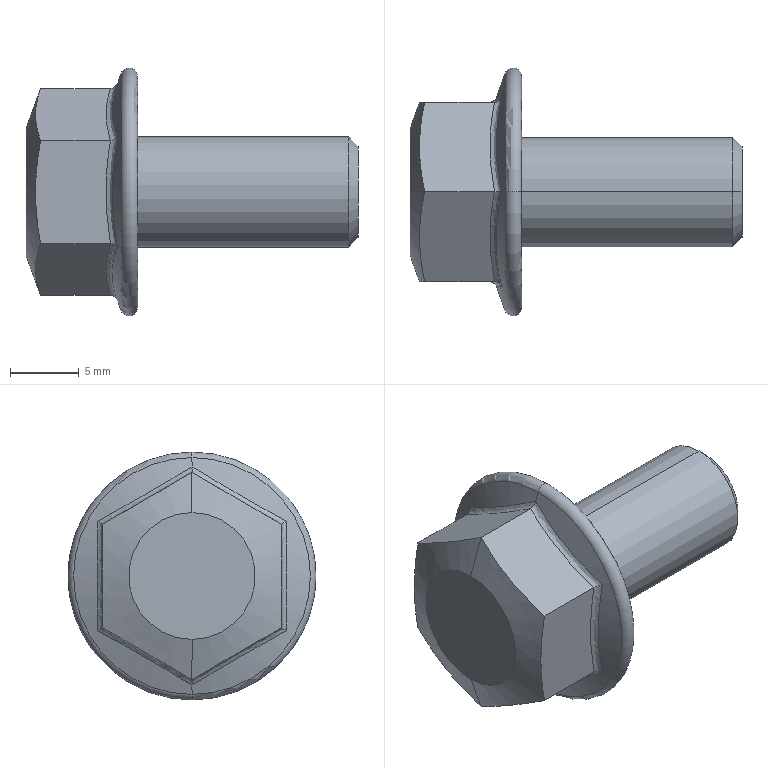Part | SolidWorks | features BaseBody 1 | 1 solid | 25 faces | box 24.1 x 18 x 18 mm | volume 2099 mm3 | plane 9 | cone 6 | spline 6 | torus 2 | cylinder 2 | commonest cylinder face diameters 8 x2
STEP:
#1=CARTESIAN_POINT('',(24.1,0.,-3.324));
#2=VERTEX_POINT('',#1);
#3=CARTESIAN_POINT('',(24.1,0.,3.324));
#4=VERTEX_POINT('',#3);
#5=CARTESIAN_POINT('',(24.1,0.,0.));
#6=DIRECTION('',(1.,0.,0.));
#7=DIRECTION('',(0.,0.,-1.));
#8=AXIS2_PLACEMENT_3D('',#5,#6,#7);
#9=CIRCLE('',#8,3.324);
#10=EDGE_CURVE('',#2,#4,#9,.T.);
#11=ORIENTED_EDGE('',*,*,#10,.F.);
#12=CARTESIAN_POINT('',(23.424,0.,-4.));
#13=VERTEX_POINT('',#12);
#14=CARTESIAN_POINT('',(24.1,0.,-3.324));
#15=DIRECTION('',(-0.7071,0.,-0.7071));
#16=VECTOR('',#15,1000.);
#17=LINE('',#14,#16);
#18=EDGE_CURVE('',#2,#13,#17,.T.);
#19=ORIENTED_EDGE('',*,*,#18,.T.);
#20=CARTESIAN_POINT('',(23.424,0.,4.));
#21=VERTEX_POINT('',#20);
#22=CARTESIAN_POINT('',(23.424,0.,0.));
#23=DIRECTION('',(-1.,0.,0.));
#24=DIRECTION('',(0.,0.,-1.));
#25=AXIS2_PLACEMENT_3D('',#22,#23,#24);
#26=CIRCLE('',#25,4.);
#27=EDGE_CURVE('',#21,#13,#26,.T.);
#28=ORIENTED_EDGE('',*,*,#27,.F.);
#29=CARTESIAN_POINT('',(24.1,0.,3.324));
#30=DIRECTION('',(-0.7071,0.,0.7071));
#31=VECTOR('',#30,1000.);
#32=LINE('',#29,#31);
#33=EDGE_CURVE('',#4,#21,#32,.T.);
#34=ORIENTED_EDGE('',*,*,#33,.F.);
#35=EDGE_LOOP('',(#11,#19,#28,#34));
#36=FACE_OUTER_BOUND('',#35,.T.);
#37=CARTESIAN_POINT('',(24.1,0.,0.));
#38=DIRECTION('',(-1.,0.,0.));
#39=DIRECTION('',(0.,0.,1.));
#40=AXIS2_PLACEMENT_3D('',#37,#38,#39);
#41=CONICAL_SURFACE('',#40,3.324,0.7854);
#42=ADVANCED_FACE('',(#36),#41,.T.);
#43=CARTESIAN_POINT('',(0.,0.,4.6));
#44=VERTEX_POINT('',#43);
#45=CARTESIAN_POINT('',(0.,0.,-4.6));
#46=VERTEX_POINT('',#45);
#47=CARTESIAN_POINT('',(0.,0.,0.));
#48=DIRECTION('',(-1.,0.,0.));
#49=DIRECTION('',(0.,0.,1.));
#50=AXIS2_PLACEMENT_3D('',#47,#48,#49);
#51=CIRCLE('',#50,4.6);
#52=EDGE_CURVE('',#44,#46,#51,.T.);
#53=ORIENTED_EDGE('',*,*,#52,.F.);
#54=CARTESIAN_POINT('',(1.058,0.,7.506));
#55=VERTEX_POINT('',#54);
#56=CARTESIAN_POINT('',(0.,0.,4.6));
#57=DIRECTION('',(0.342,0.,0.9397));
#58=VECTOR('',#57,1000.);
#59=LINE('',#56,#58);
#60=EDGE_CURVE('',#44,#55,#59,.T.);
#61=ORIENTED_EDGE('',*,*,#60,.T.);
#62=CARTESIAN_POINT('',(1.058,6.5,3.753));
#63=VERTEX_POINT('',#62);
#64=CARTESIAN_POINT('',(1.058,0.,7.506));
#65=CARTESIAN_POINT('',(0.9987,0.28,7.344));
#66=CARTESIAN_POINT('',(0.9468,0.5536,7.186));
#67=CARTESIAN_POINT('',(0.8795,0.9584,6.952));
#68=CARTESIAN_POINT('',(0.8588,1.092,6.875));
#69=CARTESIAN_POINT('',(0.8303,1.293,6.759));
#70=CARTESIAN_POINT('',(0.8213,1.359,6.721));
#71=CARTESIAN_POINT('',(0.8041,1.492,6.644));
#72=CARTESIAN_POINT('',(0.7961,1.557,6.607));
#73=CARTESIAN_POINT('',(0.7722,1.762,6.489));
#74=CARTESIAN_POINT('',(0.7583,1.897,6.41));
#75=CARTESIAN_POINT('',(0.7342,2.168,6.254));
#76=CARTESIAN_POINT('',(0.7242,2.301,6.177));
#77=CARTESIAN_POINT('',(0.6997,2.71,5.941));
#78=CARTESIAN_POINT('',(0.6915,2.979,5.786));
#79=CARTESIAN_POINT('',(0.6915,3.386,5.551));
#80=CARTESIAN_POINT('',(0.6936,3.521,5.473));
#81=CARTESIAN_POINT('',(0.7018,3.791,5.317));
#82=CARTESIAN_POINT('',(0.708,3.927,5.238));
#83=CARTESIAN_POINT('',(0.7242,4.198,5.082));
#84=CARTESIAN_POINT('',(0.7342,4.332,5.004));
#85=CARTESIAN_POINT('',(0.7523,4.535,4.887));
#86=CARTESIAN_POINT('',(0.7588,4.603,4.848));
#87=CARTESIAN_POINT('',(0.7727,4.739,4.77));
#88=CARTESIAN_POINT('',(0.7804,4.809,4.729));
#89=CARTESIAN_POINT('',(0.8501,5.406,4.384));
#90=CARTESIAN_POINT('',(0.9398,5.94,4.076));
#91=CARTESIAN_POINT('',(1.058,6.5,3.753));
#92=B_SPLINE_CURVE_WITH_KNOTS('',3,(#64,#65,#66,#67,#68,#69,#70,#71,#72,#73,#74,#75,#76,#77,#78,#79,#80,#81,#82,#83,#84,#85,#86,#87,#88,#89,#90,#91),.UNSPECIFIED.,.F.,.F.,(4,2,2,2,2,2,2,2,2,2,2,2,2,4),(0.,0.125,0.1875,0.2187,0.25,0.3125,0.375,0.5,0.5625,0.625,0.6875,0.7187,0.75,1.),.UNSPECIFIED.);
#93=EDGE_CURVE('',#55,#63,#92,.T.);
#94=ORIENTED_EDGE('',*,*,#93,.T.);
#95=CARTESIAN_POINT('',(1.058,6.5,-3.753));
#96=VERTEX_POINT('',#95);
#97=CARTESIAN_POINT('',(1.058,6.5,3.753));
#98=CARTESIAN_POINT('',(0.9989,6.5,3.43));
#99=CARTESIAN_POINT('',(0.9471,6.5,3.115));
#100=CARTESIAN_POINT('',(0.8799,6.5,2.649));
#101=CARTESIAN_POINT('',(0.8592,6.5,2.495));
#102=CARTESIAN_POINT('',(0.8308,6.5,2.264));
#103=CARTESIAN_POINT('',(0.8172,6.5,2.149));
#104=CARTESIAN_POINT('',(0.8047,6.5,2.034));
#105=CARTESIAN_POINT('',(0.7965,6.5,1.958));
#106=CARTESIAN_POINT('',(0.7926,6.5,1.921));
#107=CARTESIAN_POINT('',(0.7727,6.5,1.724));
#108=CARTESIAN_POINT('',(0.7587,6.5,1.567));
#109=CARTESIAN_POINT('',(0.7346,6.5,1.255));
#110=CARTESIAN_POINT('',(0.7246,6.5,1.101));
#111=CARTESIAN_POINT('',(0.6999,6.5,0.6296));
#112=CARTESIAN_POINT('',(0.6916,6.5,0.3193));
#113=CARTESIAN_POINT('',(0.6914,6.5,-0.3076));
#114=CARTESIAN_POINT('',(0.6997,6.5,-0.6209));
#115=CARTESIAN_POINT('',(0.7239,6.5,-1.09));
#116=CARTESIAN_POINT('',(0.734,6.5,-1.246));
#117=CARTESIAN_POINT('',(0.752,6.5,-1.481));
#118=CARTESIAN_POINT('',(0.7617,6.5,-1.598));
#119=CARTESIAN_POINT('',(0.7726,6.5,-1.716));
#120=CARTESIAN_POINT('',(0.7801,6.5,-1.795));
#121=CARTESIAN_POINT('',(0.784,6.5,-1.836));
#122=CARTESIAN_POINT('',(0.8498,6.5,-2.488));
#123=CARTESIAN_POINT('',(0.9397,6.5,-3.105));
#124=CARTESIAN_POINT('',(1.058,6.5,-3.753));
#125=B_SPLINE_CURVE_WITH_KNOTS('',3,(#97,#98,#99,#100,#101,#102,#103,#104,#105,#106,#107,#108,#109,#110,#111,#112,#113,#114,#115,#116,#117,#118,#119,#120,#121,#122,#123,#124),.UNSPECIFIED.,.F.,.F.,(4,2,2,1,2,2,2,2,2,2,2,1,2,2,4),(0.,0.125,0.1875,0.2188,0.2344,0.25,0.3125,0.375,0.5,0.625,0.6875,0.7188,0.7344,0.75,1.),.UNSPECIFIED.);
#126=EDGE_CURVE('',#63,#96,#125,.T.);
#127=ORIENTED_EDGE('',*,*,#126,.T.);
#128=CARTESIAN_POINT('',(1.058,0.,-7.506));
#129=VERTEX_POINT('',#128);
#130=CARTESIAN_POINT('',(1.058,6.5,-3.753));
#131=CARTESIAN_POINT('',(0.9987,6.22,-3.914));
#132=CARTESIAN_POINT('',(0.9468,5.946,-4.072));
#133=CARTESIAN_POINT('',(0.8795,5.541,-4.306));
#134=CARTESIAN_POINT('',(0.8588,5.408,-4.383));
#135=CARTESIAN_POINT('',(0.8303,5.207,-4.499));
#136=CARTESIAN_POINT('',(0.8213,5.141,-4.537));
#137=CARTESIAN_POINT('',(0.8041,5.008,-4.614));
#138=CARTESIAN_POINT('',(0.7961,4.943,-4.652));
#139=CARTESIAN_POINT('',(0.7722,4.738,-4.77));
#140=CARTESIAN_POINT('',(0.7583,4.603,-4.848));
#141=CARTESIAN_POINT('',(0.7342,4.332,-5.004));
#142=CARTESIAN_POINT('',(0.7242,4.199,-5.081));
#143=CARTESIAN_POINT('',(0.6997,3.79,-5.317));
#144=CARTESIAN_POINT('',(0.6915,3.521,-5.473));
#145=CARTESIAN_POINT('',(0.6915,3.114,-5.707));
#146=CARTESIAN_POINT('',(0.6936,2.979,-5.785));
#147=CARTESIAN_POINT('',(0.7018,2.709,-5.941));
#148=CARTESIAN_POINT('',(0.708,2.573,-6.02));
#149=CARTESIAN_POINT('',(0.7242,2.302,-6.176));
#150=CARTESIAN_POINT('',(0.7342,2.168,-6.254));
#151=CARTESIAN_POINT('',(0.7523,1.965,-6.371));
#152=CARTESIAN_POINT('',(0.7588,1.897,-6.41));
#153=CARTESIAN_POINT('',(0.7727,1.761,-6.489));
#154=CARTESIAN_POINT('',(0.7804,1.691,-6.529));
#155=CARTESIAN_POINT('',(0.8501,1.094,-6.874));
#156=CARTESIAN_POINT('',(0.9398,0.56,-7.182));
#157=CARTESIAN_POINT('',(1.058,0.,-7.506));
#158=B_SPLINE_CURVE_WITH_KNOTS('',3,(#130,#131,#132,#133,#134,#135,#136,#137,#138,#139,#140,#141,#142,#143,#144,#145,#146,#147,#148,#149,#150,#151,#152,#153,#154,#155,#156,#157),.UNSPECIFIED.,.F.,.F.,(4,2,2,2,2,2,2,2,2,2,2,2,2,4),(0.,0.125,0.1875,0.2187,0.25,0.3125,0.375,0.5,0.5625,0.625,0.6875,0.7187,0.75,1.),.UNSPECIFIED.);
#159=EDGE_CURVE('',#96,#129,#158,.T.);
#160=ORIENTED_EDGE('',*,*,#159,.T.);
#161=CARTESIAN_POINT('',(0.,0.,-4.6));
#162=DIRECTION('',(0.342,0.,-0.9397));
#163=VECTOR('',#162,1000.);
#164=LINE('',#161,#163);
#165=EDGE_CURVE('',#46,#129,#164,.T.);
#166=ORIENTED_EDGE('',*,*,#165,.F.);
#167=EDGE_LOOP('',(#53,#61,#94,#127,#160,#166));
#168=FACE_OUTER_BOUND('',#167,.T.);
#169=CARTESIAN_POINT('',(0.,0.,0.));
#170=DIRECTION('',(1.,0.,0.));
#171=DIRECTION('',(0.,0.,-1.));
#172=AXIS2_PLACEMENT_3D('',#169,#170,#171);
#173=CONICAL_SURFACE('',#172,4.6,1.222);
#174=ADVANCED_FACE('',(#168),#173,.T.);
#175=CARTESIAN_POINT('',(6.9,0.,-8.593));
#176=VERTEX_POINT('',#175);
#177=CARTESIAN_POINT('',(6.9,0.,8.593));
#178=VERTEX_POINT('',#177);
#179=CARTESIAN_POINT('',(6.9,0.,0.));
#180=DIRECTION('',(1.,0.,0.));
#181=DIRECTION('',(0.,0.,-1.));
#182=AXIS2_PLACEMENT_3D('',#179,#180,#181);
#183=CIRCLE('',#182,8.593);
#184=EDGE_CURVE('',#176,#178,#183,.T.);
#185=ORIENTED_EDGE('',*,*,#184,.T.);
#186=CARTESIAN_POINT('',(8.1,0.,8.381));
#187=VERTEX_POINT('',#186);
#188=CARTESIAN_POINT('',(7.481,0.,8.381));
#189=DIRECTION('',(0.,1.,0.));
#190=DIRECTION('',(0.,0.,1.));
#191=AXIS2_PLACEMENT_3D('',#188,#189,#190);
#192=CIRCLE('',#191,0.6187);
#193=EDGE_CURVE('',#178,#187,#192,.T.);
#194=ORIENTED_EDGE('',*,*,#193,.T.);
#195=CARTESIAN_POINT('',(8.1,0.,-8.381));
#196=VERTEX_POINT('',#195);
#197=CARTESIAN_POINT('',(8.1,0.,0.));
#198=DIRECTION('',(1.,0.,0.));
#199=DIRECTION('',(0.,0.,-1.));
#200=AXIS2_PLACEMENT_3D('',#197,#198,#199);
#201=CIRCLE('',#200,8.381);
#202=EDGE_CURVE('',#196,#187,#201,.T.);
#203=ORIENTED_EDGE('',*,*,#202,.F.);
#204=CARTESIAN_POINT('',(7.481,0.,-8.381));
#205=DIRECTION('',(0.,-1.,0.));
#206=DIRECTION('',(0.,0.,-1.));
#207=AXIS2_PLACEMENT_3D('',#204,#205,#206);
#208=CIRCLE('',#207,0.6187);
#209=EDGE_CURVE('',#176,#196,#208,.T.);
#210=ORIENTED_EDGE('',*,*,#209,.F.);
#211=EDGE_LOOP('',(#185,#194,#203,#210));
#212=FACE_OUTER_BOUND('',#211,.T.);
#213=CARTESIAN_POINT('',(7.481,0.,0.));
#214=DIRECTION('',(1.,0.,0.));
#215=DIRECTION('',(0.,0.,-1.));
#216=AXIS2_PLACEMENT_3D('',#213,#214,#215);
#217=TOROIDAL_SURFACE('',#216,8.381,0.6187);
#218=ADVANCED_FACE('',(#212),#217,.T.);
#219=CARTESIAN_POINT('',(6.652,6.852,3.956));
#220=VERTEX_POINT('',#219);
#221=CARTESIAN_POINT('',(6.652,0.,7.912));
#222=VERTEX_POINT('',#221);
#223=CARTESIAN_POINT('',(6.652,6.852,3.956));
#224=CARTESIAN_POINT('',(6.589,6.556,4.123));
#225=CARTESIAN_POINT('',(6.534,6.268,4.286));
#226=CARTESIAN_POINT('',(6.462,5.842,4.527));
#227=CARTESIAN_POINT('',(6.44,5.701,4.607));
#228=CARTESIAN_POINT('',(6.409,5.49,4.727));
#229=CARTESIAN_POINT('',(6.395,5.385,4.787));
#230=CARTESIAN_POINT('',(6.381,5.281,4.846));
#231=CARTESIAN_POINT('',(6.372,5.211,4.886));
#232=CARTESIAN_POINT('',(6.368,5.178,4.904));
#233=CARTESIAN_POINT('',(6.329,4.847,5.093));
#234=CARTESIAN_POINT('',(6.302,4.56,5.256));
#235=CARTESIAN_POINT('',(6.267,3.989,5.582));
#236=CARTESIAN_POINT('',(6.258,3.708,5.745));
#237=CARTESIAN_POINT('',(6.258,3.131,6.078));
#238=CARTESIAN_POINT('',(6.267,2.847,6.242));
#239=CARTESIAN_POINT('',(6.293,2.42,6.49));
#240=CARTESIAN_POINT('',(6.304,2.277,6.574));
#241=CARTESIAN_POINT('',(6.324,2.062,6.7));
#242=CARTESIAN_POINT('',(6.334,1.954,6.763));
#243=CARTESIAN_POINT('',(6.346,1.845,6.827));
#244=CARTESIAN_POINT('',(6.355,1.772,6.869));
#245=CARTESIAN_POINT('',(6.359,1.734,6.892));
#246=CARTESIAN_POINT('',(6.43,1.145,7.237));
#247=CARTESIAN_POINT('',(6.526,0.587,7.566));
#248=CARTESIAN_POINT('',(6.652,0.,7.912));
#249=B_SPLINE_CURVE_WITH_KNOTS('',3,(#223,#224,#225,#226,#227,#228,#229,#230,#231,#232,#233,#234,#235,#236,#237,#238,#239,#240,#241,#242,#243,#244,#245,#246,#247,#248),.UNSPECIFIED.,.F.,.F.,(4,2,2,1,2,2,2,2,2,2,1,2,2,4),(0.,0.125,0.1875,0.2187,0.2344,0.25,0.375,0.5,0.625,0.6875,0.7187,0.7344,0.75,1.),.UNSPECIFIED.);
#250=EDGE_CURVE('',#220,#222,#249,.T.);
#251=ORIENTED_EDGE('',*,*,#250,.T.);
#252=CARTESIAN_POINT('',(6.9,0.,8.593));
#253=DIRECTION('',(0.342,0.,0.9397));
#254=VECTOR('',#253,1000.);
#255=LINE('',#252,#254);
#256=EDGE_CURVE('',#222,#178,#255,.T.);
#257=ORIENTED_EDGE('',*,*,#256,.T.);
#258=ORIENTED_EDGE('',*,*,#184,.F.);
#259=CARTESIAN_POINT('',(6.652,0.,-7.912));
#260=VERTEX_POINT('',#259);
#261=CARTESIAN_POINT('',(6.9,0.,-8.593));
#262=DIRECTION('',(0.342,0.,-0.9397));
#263=VECTOR('',#262,1000.);
#264=LINE('',#261,#263);
#265=EDGE_CURVE('',#260,#176,#264,.T.);
#266=ORIENTED_EDGE('',*,*,#265,.F.);
#267=CARTESIAN_POINT('',(6.652,6.852,-3.956));
#268=VERTEX_POINT('',#267);
#269=CARTESIAN_POINT('',(6.652,0.,-7.912));
#270=CARTESIAN_POINT('',(6.589,0.2923,-7.739));
#271=CARTESIAN_POINT('',(6.534,0.5778,-7.571));
#272=CARTESIAN_POINT('',(6.462,1.,-7.323));
#273=CARTESIAN_POINT('',(6.44,1.14,-7.241));
#274=CARTESIAN_POINT('',(6.409,1.348,-7.118));
#275=CARTESIAN_POINT('',(6.395,1.453,-7.057));
#276=CARTESIAN_POINT('',(6.381,1.556,-6.996));
#277=CARTESIAN_POINT('',(6.372,1.626,-6.956));
#278=CARTESIAN_POINT('',(6.368,1.658,-6.937));
#279=CARTESIAN_POINT('',(6.329,1.987,-6.744));
#280=CARTESIAN_POINT('',(6.302,2.272,-6.577));
#281=CARTESIAN_POINT('',(6.267,2.84,-6.246));
#282=CARTESIAN_POINT('',(6.258,3.121,-6.083));
#283=CARTESIAN_POINT('',(6.258,3.698,-5.75));
#284=CARTESIAN_POINT('',(6.267,3.982,-5.586));
#285=CARTESIAN_POINT('',(6.293,4.411,-5.341));
#286=CARTESIAN_POINT('',(6.304,4.554,-5.259));
#287=CARTESIAN_POINT('',(6.324,4.771,-5.135));
#288=CARTESIAN_POINT('',(6.334,4.88,-5.074));
#289=CARTESIAN_POINT('',(6.346,4.99,-5.011));
#290=CARTESIAN_POINT('',(6.355,5.063,-4.97));
#291=CARTESIAN_POINT('',(6.359,5.102,-4.948));
#292=CARTESIAN_POINT('',(6.43,5.695,-4.61));
#293=CARTESIAN_POINT('',(6.526,6.259,-4.291));
#294=CARTESIAN_POINT('',(6.652,6.852,-3.956));
#295=B_SPLINE_CURVE_WITH_KNOTS('',3,(#269,#270,#271,#272,#273,#274,#275,#276,#277,#278,#279,#280,#281,#282,#283,#284,#285,#286,#287,#288,#289,#290,#291,#292,#293,#294),.UNSPECIFIED.,.F.,.F.,(4,2,2,1,2,2,2,2,2,2,1,2,2,4),(0.,0.125,0.1875,0.2188,0.2344,0.25,0.375,0.5,0.625,0.6875,0.7188,0.7344,0.75,1.),.UNSPECIFIED.);
#296=EDGE_CURVE('',#260,#268,#295,.T.);
#297=ORIENTED_EDGE('',*,*,#296,.T.);
#298=CARTESIAN_POINT('',(6.652,6.852,-3.956));
#299=CARTESIAN_POINT('',(6.589,6.849,-3.617));
#300=CARTESIAN_POINT('',(6.534,6.846,-3.285));
#301=CARTESIAN_POINT('',(6.462,6.842,-2.795));
#302=CARTESIAN_POINT('',(6.44,6.84,-2.633));
#303=CARTESIAN_POINT('',(6.409,6.839,-2.391));
#304=CARTESIAN_POINT('',(6.395,6.838,-2.271));
#305=CARTESIAN_POINT('',(6.381,6.837,-2.15));
#306=CARTESIAN_POINT('',(6.372,6.837,-2.07));
#307=CARTESIAN_POINT('',(6.368,6.836,-2.032));
#308=CARTESIAN_POINT('',(6.329,6.834,-1.651));
#309=CARTESIAN_POINT('',(6.302,6.832,-1.321));
#310=CARTESIAN_POINT('',(6.267,6.829,-0.6638));
#311=CARTESIAN_POINT('',(6.258,6.829,-0.3385));
#312=CARTESIAN_POINT('',(6.258,6.829,0.3277));
#313=CARTESIAN_POINT('',(6.267,6.829,0.6555));
#314=CARTESIAN_POINT('',(6.293,6.831,1.15));
#315=CARTESIAN_POINT('',(6.304,6.832,1.315));
#316=CARTESIAN_POINT('',(6.324,6.833,1.564));
#317=CARTESIAN_POINT('',(6.334,6.834,1.689));
#318=CARTESIAN_POINT('',(6.346,6.835,1.815));
#319=CARTESIAN_POINT('',(6.355,6.835,1.9));
#320=CARTESIAN_POINT('',(6.359,6.836,1.944));
#321=CARTESIAN_POINT('',(6.43,6.84,2.627));
#322=CARTESIAN_POINT('',(6.526,6.846,3.275));
#323=CARTESIAN_POINT('',(6.652,6.852,3.956));
#324=B_SPLINE_CURVE_WITH_KNOTS('',3,(#298,#299,#300,#301,#302,#303,#304,#305,#306,#307,#308,#309,#310,#311,#312,#313,#314,#315,#316,#317,#318,#319,#320,#321,#322,#323),.UNSPECIFIED.,.F.,.F.,(4,2,2,1,2,2,2,2,2,2,1,2,2,4),(0.,0.125,0.1875,0.2188,0.2344,0.25,0.375,0.5,0.625,0.6875,0.7188,0.7344,0.75,1.),.UNSPECIFIED.);
#325=EDGE_CURVE('',#268,#220,#324,.T.);
#326=ORIENTED_EDGE('',*,*,#325,.T.);
#327=EDGE_LOOP('',(#251,#257,#258,#266,#297,#326));
#328=FACE_OUTER_BOUND('',#327,.T.);
#329=CARTESIAN_POINT('',(6.9,0.,0.));
#330=DIRECTION('',(1.,0.,0.));
#331=DIRECTION('',(0.,0.,-1.));
#332=AXIS2_PLACEMENT_3D('',#329,#330,#331);
#333=CONICAL_SURFACE('',#332,8.593,1.222);
#334=ADVANCED_FACE('',(#328),#333,.T.);
#335=ORIENTED_EDGE('',*,*,#27,.T.);
#336=CARTESIAN_POINT('',(8.1,0.,-4.));
#337=VERTEX_POINT('',#336);
#338=CARTESIAN_POINT('',(24.1,0.,-4.));
#339=DIRECTION('',(-1.,0.,0.));
#340=VECTOR('',#339,1000.);
#341=LINE('',#338,#340);
#342=EDGE_CURVE('',#13,#337,#341,.T.);
#343=ORIENTED_EDGE('',*,*,#342,.T.);
#344=CARTESIAN_POINT('',(8.1,0.,4.));
#345=VERTEX_POINT('',#344);
#346=CARTESIAN_POINT('',(8.1,0.,0.));
#347=DIRECTION('',(1.,0.,0.));
#348=DIRECTION('',(0.,0.,-1.));
#349=AXIS2_PLACEMENT_3D('',#346,#347,#348);
#350=CIRCLE('',#349,4.);
#351=EDGE_CURVE('',#337,#345,#350,.T.);
#352=ORIENTED_EDGE('',*,*,#351,.T.);
#353=CARTESIAN_POINT('',(24.1,0.,4.));
#354=DIRECTION('',(-1.,0.,0.));
#355=VECTOR('',#354,1000.);
#356=LINE('',#353,#355);
#357=EDGE_CURVE('',#21,#345,#356,.T.);
#358=ORIENTED_EDGE('',*,*,#357,.F.);
#359=EDGE_LOOP('',(#335,#343,#352,#358));
#360=FACE_OUTER_BOUND('',#359,.T.);
#361=CARTESIAN_POINT('',(24.1,0.,0.));
#362=DIRECTION('',(-1.,0.,0.));
#363=DIRECTION('',(0.,0.,1.));
#364=AXIS2_PLACEMENT_3D('',#361,#362,#363);
#365=CYLINDRICAL_SURFACE('',#364,4.);
#366=ADVANCED_FACE('',(#360),#365,.T.);
#367=ORIENTED_EDGE('',*,*,#202,.T.);
#368=CARTESIAN_POINT('',(8.1,0.,0.));
#369=DIRECTION('',(1.,0.,0.));
#370=DIRECTION('',(0.,0.,-1.));
#371=AXIS2_PLACEMENT_3D('',#368,#369,#370);
#372=CIRCLE('',#371,8.381);
#373=EDGE_CURVE('',#187,#196,#372,.T.);
#374=ORIENTED_EDGE('',*,*,#373,.T.);
#375=EDGE_LOOP('',(#367,#374));
#376=FACE_OUTER_BOUND('',#375,.T.);
#377=CARTESIAN_POINT('',(8.1,0.,0.));
#378=DIRECTION('',(1.,0.,0.));
#379=DIRECTION('',(0.,0.,-1.));
#380=AXIS2_PLACEMENT_3D('',#377,#378,#379);
#381=CIRCLE('',#380,4.);
#382=EDGE_CURVE('',#345,#337,#381,.T.);
#383=ORIENTED_EDGE('',*,*,#382,.F.);
#384=ORIENTED_EDGE('',*,*,#351,.F.);
#385=EDGE_LOOP('',(#383,#384));
#386=FACE_BOUND('',#385,.T.);
#387=CARTESIAN_POINT('',(8.1,0.,-7.506));
#388=DIRECTION('',(1.,0.,0.));
#389=DIRECTION('',(0.,1.,0.));
#390=AXIS2_PLACEMENT_3D('',#387,#388,#389);
#391=PLANE('',#390);
#392=ADVANCED_FACE('',(#376,#386),#391,.T.);
#393=ORIENTED_EDGE('',*,*,#342,.F.);
#394=CARTESIAN_POINT('',(23.424,0.,0.));
#395=DIRECTION('',(-1.,0.,0.));
#396=DIRECTION('',(0.,0.,-1.));
#397=AXIS2_PLACEMENT_3D('',#394,#395,#396);
#398=CIRCLE('',#397,4.);
#399=EDGE_CURVE('',#13,#21,#398,.T.);
#400=ORIENTED_EDGE('',*,*,#399,.T.);
#401=ORIENTED_EDGE('',*,*,#357,.T.);
#402=ORIENTED_EDGE('',*,*,#382,.T.);
#403=EDGE_LOOP('',(#393,#400,#401,#402));
#404=FACE_OUTER_BOUND('',#403,.T.);
#405=CARTESIAN_POINT('',(24.1,0.,0.));
#406=DIRECTION('',(-1.,0.,0.));
#407=DIRECTION('',(0.,0.,1.));
#408=AXIS2_PLACEMENT_3D('',#405,#406,#407);
#409=CYLINDRICAL_SURFACE('',#408,4.);
#410=ADVANCED_FACE('',(#404),#409,.T.);
#411=CARTESIAN_POINT('',(24.1,0.,0.));
#412=DIRECTION('',(1.,0.,0.));
#413=DIRECTION('',(0.,0.,-1.));
#414=AXIS2_PLACEMENT_3D('',#411,#412,#413);
#415=CIRCLE('',#414,3.324);
#416=EDGE_CURVE('',#4,#2,#415,.T.);
#417=ORIENTED_EDGE('',*,*,#416,.T.);
#418=ORIENTED_EDGE('',*,*,#10,.T.);
#419=EDGE_LOOP('',(#417,#418));
#420=FACE_OUTER_BOUND('',#419,.T.);
#421=CARTESIAN_POINT('',(24.1,0.,0.));
#422=DIRECTION('',(1.,0.,0.));
#423=DIRECTION('',(0.,1.,0.));
#424=AXIS2_PLACEMENT_3D('',#421,#422,#423);
#425=PLANE('',#424);
#426=ADVANCED_FACE('',(#420),#425,.T.);
#427=ORIENTED_EDGE('',*,*,#256,.F.);
#428=CARTESIAN_POINT('',(6.652,-6.852,3.956));
#429=VERTEX_POINT('',#428);
#430=CARTESIAN_POINT('',(6.652,0.,7.912));
#431=CARTESIAN_POINT('',(6.589,-0.2923,7.739));
#432=CARTESIAN_POINT('',(6.534,-0.5778,7.571));
#433=CARTESIAN_POINT('',(6.462,-1.,7.323));
#434=CARTESIAN_POINT('',(6.44,-1.14,7.241));
#435=CARTESIAN_POINT('',(6.409,-1.348,7.118));
#436=CARTESIAN_POINT('',(6.395,-1.453,7.057));
#437=CARTESIAN_POINT('',(6.381,-1.556,6.996));
#438=CARTESIAN_POINT('',(6.372,-1.626,6.956));
#439=CARTESIAN_POINT('',(6.368,-1.658,6.937));
#440=CARTESIAN_POINT('',(6.329,-1.987,6.744));
#441=CARTESIAN_POINT('',(6.302,-2.272,6.577));
#442=CARTESIAN_POINT('',(6.267,-2.84,6.246));
#443=CARTESIAN_POINT('',(6.258,-3.121,6.083));
#444=CARTESIAN_POINT('',(6.258,-3.698,5.75));
#445=CARTESIAN_POINT('',(6.267,-3.982,5.586));
#446=CARTESIAN_POINT('',(6.293,-4.411,5.341));
#447=CARTESIAN_POINT('',(6.304,-4.554,5.259));
#448=CARTESIAN_POINT('',(6.324,-4.771,5.135));
#449=CARTESIAN_POINT('',(6.334,-4.88,5.074));
#450=CARTESIAN_POINT('',(6.346,-4.99,5.011));
#451=CARTESIAN_POINT('',(6.355,-5.063,4.97));
#452=CARTESIAN_POINT('',(6.359,-5.102,4.948));
#453=CARTESIAN_POINT('',(6.43,-5.695,4.61));
#454=CARTESIAN_POINT('',(6.526,-6.259,4.291));
#455=CARTESIAN_POINT('',(6.652,-6.852,3.956));
#456=B_SPLINE_CURVE_WITH_KNOTS('',3,(#430,#431,#432,#433,#434,#435,#436,#437,#438,#439,#440,#441,#442,#443,#444,#445,#446,#447,#448,#449,#450,#451,#452,#453,#454,#455),.UNSPECIFIED.,.F.,.F.,(4,2,2,1,2,2,2,2,2,2,1,2,2,4),(0.,0.125,0.1875,0.2187,0.2344,0.25,0.375,0.5,0.625,0.6875,0.7188,0.7344,0.75,1.),.UNSPECIFIED.);
#457=EDGE_CURVE('',#222,#429,#456,.T.);
#458=ORIENTED_EDGE('',*,*,#457,.T.);
#459=CARTESIAN_POINT('',(6.652,-6.852,-3.956));
#460=VERTEX_POINT('',#459);
#461=CARTESIAN_POINT('',(6.652,-6.852,3.956));
#462=CARTESIAN_POINT('',(6.589,-6.849,3.617));
#463=CARTESIAN_POINT('',(6.534,-6.846,3.285));
#464=CARTESIAN_POINT('',(6.462,-6.842,2.795));
#465=CARTESIAN_POINT('',(6.44,-6.84,2.633));
#466=CARTESIAN_POINT('',(6.409,-6.839,2.391));
#467=CARTESIAN_POINT('',(6.395,-6.838,2.271));
#468=CARTESIAN_POINT('',(6.381,-6.837,2.15));
#469=CARTESIAN_POINT('',(6.372,-6.837,2.07));
#470=CARTESIAN_POINT('',(6.368,-6.836,2.032));
#471=CARTESIAN_POINT('',(6.329,-6.834,1.651));
#472=CARTESIAN_POINT('',(6.302,-6.832,1.321));
#473=CARTESIAN_POINT('',(6.267,-6.829,0.6637));
#474=CARTESIAN_POINT('',(6.258,-6.829,0.3384));
#475=CARTESIAN_POINT('',(6.258,-6.829,-0.3278));
#476=CARTESIAN_POINT('',(6.267,-6.829,-0.6556));
#477=CARTESIAN_POINT('',(6.293,-6.831,-1.15));
#478=CARTESIAN_POINT('',(6.304,-6.832,-1.315));
#479=CARTESIAN_POINT('',(6.324,-6.833,-1.564));
#480=CARTESIAN_POINT('',(6.334,-6.834,-1.689));
#481=CARTESIAN_POINT('',(6.346,-6.835,-1.816));
#482=CARTESIAN_POINT('',(6.355,-6.835,-1.9));
#483=CARTESIAN_POINT('',(6.359,-6.836,-1.944));
#484=CARTESIAN_POINT('',(6.43,-6.84,-2.627));
#485=CARTESIAN_POINT('',(6.526,-6.846,-3.275));
#486=CARTESIAN_POINT('',(6.652,-6.852,-3.956));
#487=B_SPLINE_CURVE_WITH_KNOTS('',3,(#461,#462,#463,#464,#465,#466,#467,#468,#469,#470,#471,#472,#473,#474,#475,#476,#477,#478,#479,#480,#481,#482,#483,#484,#485,#486),.UNSPECIFIED.,.F.,.F.,(4,2,2,1,2,2,2,2,2,2,1,2,2,4),(0.,0.125,0.1875,0.2188,0.2344,0.25,0.375,0.5,0.625,0.6875,0.7188,0.7344,0.75,1.),.UNSPECIFIED.);
#488=EDGE_CURVE('',#429,#460,#487,.T.);
#489=ORIENTED_EDGE('',*,*,#488,.T.);
#490=CARTESIAN_POINT('',(6.652,-6.852,-3.956));
#491=CARTESIAN_POINT('',(6.589,-6.556,-4.123));
#492=CARTESIAN_POINT('',(6.534,-6.268,-4.286));
#493=CARTESIAN_POINT('',(6.462,-5.842,-4.527));
#494=CARTESIAN_POINT('',(6.44,-5.701,-4.607));
#495=CARTESIAN_POINT('',(6.409,-5.49,-4.727));
#496=CARTESIAN_POINT('',(6.395,-5.385,-4.787));
#497=CARTESIAN_POINT('',(6.381,-5.281,-4.846));
#498=CARTESIAN_POINT('',(6.372,-5.211,-4.886));
#499=CARTESIAN_POINT('',(6.368,-5.178,-4.904));
#500=CARTESIAN_POINT('',(6.329,-4.847,-5.093));
#501=CARTESIAN_POINT('',(6.302,-4.56,-5.256));
#502=CARTESIAN_POINT('',(6.267,-3.989,-5.582));
#503=CARTESIAN_POINT('',(6.258,-3.708,-5.745));
#504=CARTESIAN_POINT('',(6.258,-3.131,-6.078));
#505=CARTESIAN_POINT('',(6.267,-2.847,-6.242));
#506=CARTESIAN_POINT('',(6.293,-2.42,-6.49));
#507=CARTESIAN_POINT('',(6.304,-2.277,-6.574));
#508=CARTESIAN_POINT('',(6.324,-2.062,-6.7));
#509=CARTESIAN_POINT('',(6.334,-1.954,-6.763));
#510=CARTESIAN_POINT('',(6.346,-1.845,-6.827));
#511=CARTESIAN_POINT('',(6.355,-1.772,-6.869));
#512=CARTESIAN_POINT('',(6.359,-1.734,-6.892));
#513=CARTESIAN_POINT('',(6.43,-1.145,-7.237));
#514=CARTESIAN_POINT('',(6.526,-0.587,-7.566));
#515=CARTESIAN_POINT('',(6.652,0.,-7.912));
#516=B_SPLINE_CURVE_WITH_KNOTS('',3,(#490,#491,#492,#493,#494,#495,#496,#497,#498,#499,#500,#501,#502,#503,#504,#505,#506,#507,#508,#509,#510,#511,#512,#513,#514,#515),.UNSPECIFIED.,.F.,.F.,(4,2,2,1,2,2,2,2,2,2,1,2,2,4),(0.,0.125,0.1875,0.2188,0.2344,0.25,0.375,0.5,0.625,0.6875,0.7187,0.7344,0.75,1.),.UNSPECIFIED.);
#517=EDGE_CURVE('',#460,#260,#516,.T.);
#518=ORIENTED_EDGE('',*,*,#517,.T.);
#519=ORIENTED_EDGE('',*,*,#265,.T.);
#520=CARTESIAN_POINT('',(6.9,0.,0.));
#521=DIRECTION('',(1.,0.,0.));
#522=DIRECTION('',(0.,0.,-1.));
#523=AXIS2_PLACEMENT_3D('',#520,#521,#522);
#524=CIRCLE('',#523,8.593);
#525=EDGE_CURVE('',#178,#176,#524,.T.);
#526=ORIENTED_EDGE('',*,*,#525,.F.);
#527=EDGE_LOOP('',(#427,#458,#489,#518,#519,#526));
#528=FACE_OUTER_BOUND('',#527,.T.);
#529=CARTESIAN_POINT('',(6.9,0.,0.));
#530=DIRECTION('',(1.,0.,0.));
#531=DIRECTION('',(0.,0.,-1.));
#532=AXIS2_PLACEMENT_3D('',#529,#530,#531);
#533=CONICAL_SURFACE('',#532,8.593,1.222);
#534=ADVANCED_FACE('',(#528),#533,.T.);
#535=ORIENTED_EDGE('',*,*,#193,.F.);
#536=ORIENTED_EDGE('',*,*,#525,.T.);
#537=ORIENTED_EDGE('',*,*,#209,.T.);
#538=ORIENTED_EDGE('',*,*,#373,.F.);
#539=EDGE_LOOP('',(#535,#536,#537,#538));
#540=FACE_OUTER_BOUND('',#539,.T.);
#541=CARTESIAN_POINT('',(7.481,0.,0.));
#542=DIRECTION('',(1.,0.,0.));
#543=DIRECTION('',(0.,0.,-1.));
#544=AXIS2_PLACEMENT_3D('',#541,#542,#543);
#545=TOROIDAL_SURFACE('',#544,8.381,0.6187);
#546=ADVANCED_FACE('',(#540),#545,.T.);
#547=CARTESIAN_POINT('',(0.,0.,0.));
#548=DIRECTION('',(-1.,0.,0.));
#549=DIRECTION('',(0.,0.,1.));
#550=AXIS2_PLACEMENT_3D('',#547,#548,#549);
#551=CIRCLE('',#550,4.6);
#552=EDGE_CURVE('',#46,#44,#551,.T.);
#553=ORIENTED_EDGE('',*,*,#552,.T.);
#554=ORIENTED_EDGE('',*,*,#52,.T.);
#555=EDGE_LOOP('',(#553,#554));
#556=FACE_OUTER_BOUND('',#555,.T.);
#557=CARTESIAN_POINT('',(0.,0.,-7.506));
#558=DIRECTION('',(1.,0.,0.));
#559=DIRECTION('',(0.,1.,0.));
#560=AXIS2_PLACEMENT_3D('',#557,#558,#559);
#561=PLANE('',#560);
#562=ADVANCED_FACE('',(#556),#561,.F.);
#563=ORIENTED_EDGE('',*,*,#60,.F.);
#564=ORIENTED_EDGE('',*,*,#552,.F.);
#565=ORIENTED_EDGE('',*,*,#165,.T.);
#566=CARTESIAN_POINT('',(1.058,-6.5,-3.753));
#567=VERTEX_POINT('',#566);
#568=CARTESIAN_POINT('',(1.058,0.,-7.506));
#569=CARTESIAN_POINT('',(0.9987,-0.28,-7.344));
#570=CARTESIAN_POINT('',(0.9468,-0.5536,-7.186));
#571=CARTESIAN_POINT('',(0.8795,-0.9584,-6.952));
#572=CARTESIAN_POINT('',(0.8588,-1.092,-6.875));
#573=CARTESIAN_POINT('',(0.8303,-1.293,-6.759));
#574=CARTESIAN_POINT('',(0.8213,-1.359,-6.721));
#575=CARTESIAN_POINT('',(0.8041,-1.492,-6.644));
#576=CARTESIAN_POINT('',(0.7961,-1.557,-6.607));
#577=CARTESIAN_POINT('',(0.7722,-1.762,-6.489));
#578=CARTESIAN_POINT('',(0.7583,-1.897,-6.41));
#579=CARTESIAN_POINT('',(0.7342,-2.168,-6.254));
#580=CARTESIAN_POINT('',(0.7242,-2.301,-6.177));
#581=CARTESIAN_POINT('',(0.6997,-2.71,-5.941));
#582=CARTESIAN_POINT('',(0.6915,-2.979,-5.786));
#583=CARTESIAN_POINT('',(0.6915,-3.386,-5.551));
#584=CARTESIAN_POINT('',(0.6936,-3.521,-5.473));
#585=CARTESIAN_POINT('',(0.7018,-3.791,-5.317));
#586=CARTESIAN_POINT('',(0.708,-3.927,-5.238));
#587=CARTESIAN_POINT('',(0.7242,-4.198,-5.082));
#588=CARTESIAN_POINT('',(0.7342,-4.332,-5.004));
#589=CARTESIAN_POINT('',(0.7523,-4.535,-4.887));
#590=CARTESIAN_POINT('',(0.7588,-4.603,-4.848));
#591=CARTESIAN_POINT('',(0.7727,-4.739,-4.77));
#592=CARTESIAN_POINT('',(0.7804,-4.809,-4.729));
#593=CARTESIAN_POINT('',(0.8501,-5.406,-4.384));
#594=CARTESIAN_POINT('',(0.9398,-5.94,-4.076));
#595=CARTESIAN_POINT('',(1.058,-6.5,-3.753));
#596=B_SPLINE_CURVE_WITH_KNOTS('',3,(#568,#569,#570,#571,#572,#573,#574,#575,#576,#577,#578,#579,#580,#581,#582,#583,#584,#585,#586,#587,#588,#589,#590,#591,#592,#593,#594,#595),.UNSPECIFIED.,.F.,.F.,(4,2,2,2,2,2,2,2,2,2,2,2,2,4),(0.,0.125,0.1875,0.2188,0.25,0.3125,0.375,0.5,0.5625,0.625,0.6875,0.7187,0.75,1.),.UNSPECIFIED.);
#597=EDGE_CURVE('',#129,#567,#596,.T.);
#598=ORIENTED_EDGE('',*,*,#597,.T.);
#599=CARTESIAN_POINT('',(1.058,-6.5,3.753));
#600=VERTEX_POINT('',#599);
#601=CARTESIAN_POINT('',(1.058,-6.5,-3.753));
#602=CARTESIAN_POINT('',(0.9986,-6.5,-3.429));
#603=CARTESIAN_POINT('',(0.9467,-6.5,-3.113));
#604=CARTESIAN_POINT('',(0.8793,-6.5,-2.645));
#605=CARTESIAN_POINT('',(0.8586,-6.5,-2.49));
#606=CARTESIAN_POINT('',(0.8301,-6.5,-2.258));
#607=CARTESIAN_POINT('',(0.8165,-6.5,-2.143));
#608=CARTESIAN_POINT('',(0.8039,-6.5,-2.028));
#609=CARTESIAN_POINT('',(0.7958,-6.5,-1.951));
#610=CARTESIAN_POINT('',(0.7919,-6.5,-1.914));
#611=CARTESIAN_POINT('',(0.756,-6.5,-1.558));
#612=CARTESIAN_POINT('',(0.7321,-6.5,-1.248));
#613=CARTESIAN_POINT('',(0.6995,-6.5,-0.6187));
#614=CARTESIAN_POINT('',(0.6914,-6.5,-0.3072));
#615=CARTESIAN_POINT('',(0.6916,-6.5,0.1624));
#616=CARTESIAN_POINT('',(0.6937,-6.5,0.3183));
#617=CARTESIAN_POINT('',(0.702,-6.5,0.6305));
#618=CARTESIAN_POINT('',(0.7082,-6.5,0.7883));
#619=CARTESIAN_POINT('',(0.7245,-6.5,1.1));
#620=CARTESIAN_POINT('',(0.7346,-6.5,1.255));
#621=CARTESIAN_POINT('',(0.7527,-6.5,1.489));
#622=CARTESIAN_POINT('',(0.7625,-6.5,1.607));
#623=CARTESIAN_POINT('',(0.7733,-6.5,1.724));
#624=CARTESIAN_POINT('',(0.7808,-6.5,1.803));
#625=CARTESIAN_POINT('',(0.7848,-6.5,1.843));
#626=CARTESIAN_POINT('',(0.8505,-6.5,2.493));
#627=CARTESIAN_POINT('',(0.9402,-6.5,3.108));
#628=CARTESIAN_POINT('',(1.058,-6.5,3.753));
#629=B_SPLINE_CURVE_WITH_KNOTS('',3,(#601,#602,#603,#604,#605,#606,#607,#608,#609,#610,#611,#612,#613,#614,#615,#616,#617,#618,#619,#620,#621,#622,#623,#624,#625,#626,#627,#628),.UNSPECIFIED.,.F.,.F.,(4,2,2,1,2,2,2,2,2,2,2,1,2,2,4),(0.,0.125,0.1875,0.2188,0.2344,0.25,0.375,0.5,0.5625,0.625,0.6875,0.7188,0.7344,0.75,1.),.UNSPECIFIED.);
#630=EDGE_CURVE('',#567,#600,#629,.T.);
#631=ORIENTED_EDGE('',*,*,#630,.T.);
#632=CARTESIAN_POINT('',(1.058,-6.5,3.753));
#633=CARTESIAN_POINT('',(0.9987,-6.22,3.914));
#634=CARTESIAN_POINT('',(0.9468,-5.946,4.072));
#635=CARTESIAN_POINT('',(0.8795,-5.541,4.306));
#636=CARTESIAN_POINT('',(0.8588,-5.408,4.383));
#637=CARTESIAN_POINT('',(0.8303,-5.207,4.499));
#638=CARTESIAN_POINT('',(0.8213,-5.141,4.537));
#639=CARTESIAN_POINT('',(0.8041,-5.008,4.614));
#640=CARTESIAN_POINT('',(0.7961,-4.943,4.652));
#641=CARTESIAN_POINT('',(0.7722,-4.738,4.77));
#642=CARTESIAN_POINT('',(0.7583,-4.603,4.848));
#643=CARTESIAN_POINT('',(0.7342,-4.332,5.004));
#644=CARTESIAN_POINT('',(0.7242,-4.199,5.081));
#645=CARTESIAN_POINT('',(0.6997,-3.79,5.317));
#646=CARTESIAN_POINT('',(0.6915,-3.521,5.473));
#647=CARTESIAN_POINT('',(0.6915,-3.114,5.707));
#648=CARTESIAN_POINT('',(0.6936,-2.979,5.785));
#649=CARTESIAN_POINT('',(0.7018,-2.709,5.941));
#650=CARTESIAN_POINT('',(0.708,-2.573,6.02));
#651=CARTESIAN_POINT('',(0.7242,-2.302,6.176));
#652=CARTESIAN_POINT('',(0.7342,-2.168,6.254));
#653=CARTESIAN_POINT('',(0.7523,-1.965,6.371));
#654=CARTESIAN_POINT('',(0.7588,-1.897,6.41));
#655=CARTESIAN_POINT('',(0.7727,-1.761,6.489));
#656=CARTESIAN_POINT('',(0.7804,-1.691,6.529));
#657=CARTESIAN_POINT('',(0.8501,-1.094,6.874));
#658=CARTESIAN_POINT('',(0.9398,-0.56,7.182));
#659=CARTESIAN_POINT('',(1.058,0.,7.506));
#660=B_SPLINE_CURVE_WITH_KNOTS('',3,(#632,#633,#634,#635,#636,#637,#638,#639,#640,#641,#642,#643,#644,#645,#646,#647,#648,#649,#650,#651,#652,#653,#654,#655,#656,#657,#658,#659),.UNSPECIFIED.,.F.,.F.,(4,2,2,2,2,2,2,2,2,2,2,2,2,4),(0.,0.125,0.1875,0.2187,0.25,0.3125,0.375,0.5,0.5625,0.625,0.6875,0.7188,0.75,1.),.UNSPECIFIED.);
#661=EDGE_CURVE('',#600,#55,#660,.T.);
#662=ORIENTED_EDGE('',*,*,#661,.T.);
#663=EDGE_LOOP('',(#563,#564,#565,#598,#631,#662));
#664=FACE_OUTER_BOUND('',#663,.T.);
#665=CARTESIAN_POINT('',(0.,0.,0.));
#666=DIRECTION('',(1.,0.,0.));
#667=DIRECTION('',(0.,0.,-1.));
#668=AXIS2_PLACEMENT_3D('',#665,#666,#667);
#669=CONICAL_SURFACE('',#668,4.6,1.222);
#670=ADVANCED_FACE('',(#664),#669,.T.);
#671=CARTESIAN_POINT('',(6.131,-6.5,-3.753));
#672=VERTEX_POINT('',#671);
#673=CARTESIAN_POINT('',(8.1,-6.5,-3.753));
#674=DIRECTION('',(-1.,0.,0.));
#675=VECTOR('',#674,1000.);
#676=LINE('',#673,#675);
#677=EDGE_CURVE('',#672,#567,#676,.T.);
#678=ORIENTED_EDGE('',*,*,#677,.F.);
#679=CARTESIAN_POINT('',(6.131,-6.5,3.753));
#680=VERTEX_POINT('',#679);
#681=CARTESIAN_POINT('',(6.131,-6.5,-3.753));
#682=CARTESIAN_POINT('',(5.918,-6.5,-2.511));
#683=CARTESIAN_POINT('',(5.788,-6.5,-1.261));
#684=CARTESIAN_POINT('',(5.788,-6.5,1.261));
#685=CARTESIAN_POINT('',(5.918,-6.5,2.511));
#686=CARTESIAN_POINT('',(6.131,-6.5,3.753));
#687=B_SPLINE_CURVE_WITH_KNOTS('',3,(#681,#682,#683,#684,#685,#686),.UNSPECIFIED.,.F.,.F.,(4,2,4),(0.,0.003768,0.007537),.UNSPECIFIED.);
#688=EDGE_CURVE('',#672,#680,#687,.T.);
#689=ORIENTED_EDGE('',*,*,#688,.T.);
#690=CARTESIAN_POINT('',(8.1,-6.5,3.753));
#691=DIRECTION('',(-1.,0.,0.));
#692=VECTOR('',#691,1000.);
#693=LINE('',#690,#692);
#694=EDGE_CURVE('',#680,#600,#693,.T.);
#695=ORIENTED_EDGE('',*,*,#694,.T.);
#696=ORIENTED_EDGE('',*,*,#630,.F.);
#697=EDGE_LOOP('',(#678,#689,#695,#696));
#698=FACE_OUTER_BOUND('',#697,.T.);
#699=CARTESIAN_POINT('',(8.1,-6.5,3.753));
#700=DIRECTION('',(0.,1.,0.));
#701=DIRECTION('',(0.,0.,-1.));
#702=AXIS2_PLACEMENT_3D('',#699,#700,#701);
#703=PLANE('',#702);
#704=ADVANCED_FACE('',(#698),#703,.F.);
#705=ORIENTED_EDGE('',*,*,#694,.F.);
#706=CARTESIAN_POINT('',(6.131,0.,7.506));
#707=VERTEX_POINT('',#706);
#708=CARTESIAN_POINT('',(6.131,-6.5,3.753));
#709=CARTESIAN_POINT('',(5.918,-5.425,4.374));
#710=CARTESIAN_POINT('',(5.788,-4.342,4.998));
#711=CARTESIAN_POINT('',(5.788,-2.158,6.26));
#712=CARTESIAN_POINT('',(5.918,-1.075,6.885));
#713=CARTESIAN_POINT('',(6.131,0.,7.506));
#714=B_SPLINE_CURVE_WITH_KNOTS('',3,(#708,#709,#710,#711,#712,#713),.UNSPECIFIED.,.F.,.F.,(4,2,4),(0.,0.003768,0.007537),.UNSPECIFIED.);
#715=EDGE_CURVE('',#680,#707,#714,.T.);
#716=ORIENTED_EDGE('',*,*,#715,.T.);
#717=CARTESIAN_POINT('',(8.1,0.,7.506));
#718=DIRECTION('',(-1.,0.,0.));
#719=VECTOR('',#718,1000.);
#720=LINE('',#717,#719);
#721=EDGE_CURVE('',#707,#55,#720,.T.);
#722=ORIENTED_EDGE('',*,*,#721,.T.);
#723=ORIENTED_EDGE('',*,*,#661,.F.);
#724=EDGE_LOOP('',(#705,#716,#722,#723));
#725=FACE_OUTER_BOUND('',#724,.T.);
#726=CARTESIAN_POINT('',(8.1,0.,7.506));
#727=DIRECTION('',(0.,0.5,-0.866));
#728=DIRECTION('',(-1.,0.,0.));
#729=AXIS2_PLACEMENT_3D('',#726,#727,#728);
#730=PLANE('',#729);
#731=ADVANCED_FACE('',(#725),#730,.F.);
#732=ORIENTED_EDGE('',*,*,#721,.F.);
#733=CARTESIAN_POINT('',(6.131,6.5,3.753));
#734=VERTEX_POINT('',#733);
#735=CARTESIAN_POINT('',(6.131,0.,7.506));
#736=CARTESIAN_POINT('',(5.918,1.075,6.885));
#737=CARTESIAN_POINT('',(5.788,2.158,6.26));
#738=CARTESIAN_POINT('',(5.788,4.342,4.998));
#739=CARTESIAN_POINT('',(5.918,5.425,4.374));
#740=CARTESIAN_POINT('',(6.131,6.5,3.753));
#741=B_SPLINE_CURVE_WITH_KNOTS('',3,(#735,#736,#737,#738,#739,#740),.UNSPECIFIED.,.F.,.F.,(4,2,4),(0.,0.003768,0.007537),.UNSPECIFIED.);
#742=EDGE_CURVE('',#707,#734,#741,.T.);
#743=ORIENTED_EDGE('',*,*,#742,.T.);
#744=CARTESIAN_POINT('',(8.1,6.5,3.753));
#745=DIRECTION('',(-1.,0.,0.));
#746=VECTOR('',#745,1000.);
#747=LINE('',#744,#746);
#748=EDGE_CURVE('',#734,#63,#747,.T.);
#749=ORIENTED_EDGE('',*,*,#748,.T.);
#750=ORIENTED_EDGE('',*,*,#93,.F.);
#751=EDGE_LOOP('',(#732,#743,#749,#750));
#752=FACE_OUTER_BOUND('',#751,.T.);
#753=CARTESIAN_POINT('',(8.1,6.5,3.753));
#754=DIRECTION('',(0.,-0.5,-0.866));
#755=DIRECTION('',(0.,-0.866,0.5));
#756=AXIS2_PLACEMENT_3D('',#753,#754,#755);
#757=PLANE('',#756);
#758=ADVANCED_FACE('',(#752),#757,.F.);
#759=ORIENTED_EDGE('',*,*,#748,.F.);
#760=CARTESIAN_POINT('',(6.131,6.5,-3.753));
#761=VERTEX_POINT('',#760);
#762=CARTESIAN_POINT('',(6.131,6.5,3.753));
#763=CARTESIAN_POINT('',(5.918,6.5,2.511));
#764=CARTESIAN_POINT('',(5.788,6.5,1.261));
#765=CARTESIAN_POINT('',(5.788,6.5,-1.261));
#766=CARTESIAN_POINT('',(5.918,6.5,-2.511));
#767=CARTESIAN_POINT('',(6.131,6.5,-3.753));
#768=B_SPLINE_CURVE_WITH_KNOTS('',3,(#762,#763,#764,#765,#766,#767),.UNSPECIFIED.,.F.,.F.,(4,2,4),(0.,0.003768,0.007537),.UNSPECIFIED.);
#769=EDGE_CURVE('',#734,#761,#768,.T.);
#770=ORIENTED_EDGE('',*,*,#769,.T.);
#771=CARTESIAN_POINT('',(8.1,6.5,-3.753));
#772=DIRECTION('',(-1.,0.,0.));
#773=VECTOR('',#772,1000.);
#774=LINE('',#771,#773);
#775=EDGE_CURVE('',#761,#96,#774,.T.);
#776=ORIENTED_EDGE('',*,*,#775,.T.);
#777=ORIENTED_EDGE('',*,*,#126,.F.);
#778=EDGE_LOOP('',(#759,#770,#776,#777));
#779=FACE_OUTER_BOUND('',#778,.T.);
#780=CARTESIAN_POINT('',(8.1,6.5,-3.753));
#781=DIRECTION('',(0.,-1.,0.));
#782=DIRECTION('',(0.,0.,-1.));
#783=AXIS2_PLACEMENT_3D('',#780,#781,#782);
#784=PLANE('',#783);
#785=ADVANCED_FACE('',(#779),#784,.F.);
#786=ORIENTED_EDGE('',*,*,#775,.F.);
#787=CARTESIAN_POINT('',(6.131,0.,-7.506));
#788=VERTEX_POINT('',#787);
#789=CARTESIAN_POINT('',(6.131,6.5,-3.753));
#790=CARTESIAN_POINT('',(5.918,5.425,-4.374));
#791=CARTESIAN_POINT('',(5.788,4.342,-4.998));
#792=CARTESIAN_POINT('',(5.788,2.158,-6.26));
#793=CARTESIAN_POINT('',(5.918,1.075,-6.885));
#794=CARTESIAN_POINT('',(6.131,0.,-7.506));
#795=B_SPLINE_CURVE_WITH_KNOTS('',3,(#789,#790,#791,#792,#793,#794),.UNSPECIFIED.,.F.,.F.,(4,2,4),(0.,0.003768,0.007537),.UNSPECIFIED.);
#796=EDGE_CURVE('',#761,#788,#795,.T.);
#797=ORIENTED_EDGE('',*,*,#796,.T.);
#798=CARTESIAN_POINT('',(8.1,0.,-7.506));
#799=DIRECTION('',(-1.,0.,0.));
#800=VECTOR('',#799,1000.);
#801=LINE('',#798,#800);
#802=EDGE_CURVE('',#788,#129,#801,.T.);
#803=ORIENTED_EDGE('',*,*,#802,.T.);
#804=ORIENTED_EDGE('',*,*,#159,.F.);
#805=EDGE_LOOP('',(#786,#797,#803,#804));
#806=FACE_OUTER_BOUND('',#805,.T.);
#807=CARTESIAN_POINT('',(8.1,0.,-7.506));
#808=DIRECTION('',(0.,-0.5,0.866));
#809=DIRECTION('',(-1.,0.,0.));
#810=AXIS2_PLACEMENT_3D('',#807,#808,#809);
#811=PLANE('',#810);
#812=ADVANCED_FACE('',(#806),#811,.F.);
#813=ORIENTED_EDGE('',*,*,#802,.F.);
#814=CARTESIAN_POINT('',(6.131,0.,-7.506));
#815=CARTESIAN_POINT('',(5.918,-1.075,-6.885));
#816=CARTESIAN_POINT('',(5.788,-2.158,-6.26));
#817=CARTESIAN_POINT('',(5.788,-4.342,-4.998));
#818=CARTESIAN_POINT('',(5.918,-5.425,-4.374));
#819=CARTESIAN_POINT('',(6.131,-6.5,-3.753));
#820=B_SPLINE_CURVE_WITH_KNOTS('',3,(#814,#815,#816,#817,#818,#819),.UNSPECIFIED.,.F.,.F.,(4,2,4),(0.,0.003768,0.007537),.UNSPECIFIED.);
#821=EDGE_CURVE('',#788,#672,#820,.T.);
#822=ORIENTED_EDGE('',*,*,#821,.T.);
#823=ORIENTED_EDGE('',*,*,#677,.T.);
#824=ORIENTED_EDGE('',*,*,#597,.F.);
#825=EDGE_LOOP('',(#813,#822,#823,#824));
#826=FACE_OUTER_BOUND('',#825,.T.);
#827=CARTESIAN_POINT('',(8.1,-6.5,-3.753));
#828=DIRECTION('',(0.,0.5,0.866));
#829=DIRECTION('',(1.,0.,0.));
#830=AXIS2_PLACEMENT_3D('',#827,#828,#829);
#831=PLANE('',#830);
#832=ADVANCED_FACE('',(#826),#831,.F.);
#833=CARTESIAN_POINT('',(6.652,0.,-7.912));
#834=CARTESIAN_POINT('',(6.633,0.,-7.859));
#835=CARTESIAN_POINT('',(6.605,-0.0005993,-7.805));
#836=CARTESIAN_POINT('',(6.555,0.0003018,-7.732));
#837=CARTESIAN_POINT('',(6.537,0.0002952,-7.709));
#838=CARTESIAN_POINT('',(6.507,0.0001793,-7.676));
#839=CARTESIAN_POINT('',(6.497,0.0001229,-7.666));
#840=CARTESIAN_POINT('',(6.475,0.00003051,-7.646));
#841=CARTESIAN_POINT('',(6.466,-0.00000547,-7.637));
#842=CARTESIAN_POINT('',(6.429,-0.000005802,-7.607));
#843=CARTESIAN_POINT('',(6.403,-0.00004714,-7.589));
#844=CARTESIAN_POINT('',(6.365,-0.00005987,-7.567));
#845=CARTESIAN_POINT('',(6.346,-0.00005727,-7.557));
#846=CARTESIAN_POINT('',(6.328,-0.00004764,-7.549));
#847=CARTESIAN_POINT('',(6.315,-0.00004197,-7.543));
#848=CARTESIAN_POINT('',(6.31,-0.0000396,-7.541));
#849=CARTESIAN_POINT('',(6.245,-0.00003029,-7.516));
#850=CARTESIAN_POINT('',(6.186,0.000008043,-7.506));
#851=CARTESIAN_POINT('',(6.131,0.,-7.506));
#852=B_SPLINE_CURVE_WITH_KNOTS('',3,(#833,#834,#835,#836,#837,#838,#839,#840,#841,#842,#843,#844,#845,#846,#847,#848,#849,#850,#851),.UNSPECIFIED.,.F.,.F.,(4,2,2,2,2,2,1,2,2,4),(0.,0.25,0.375,0.4375,0.5,0.625,0.6875,0.7187,0.75,1.),.UNSPECIFIED.);
#853=EDGE_CURVE('',#260,#788,#852,.T.);
#854=ORIENTED_EDGE('',*,*,#853,.F.);
#855=ORIENTED_EDGE('',*,*,#517,.F.);
#856=CARTESIAN_POINT('',(6.131,-6.5,-3.753));
#857=CARTESIAN_POINT('',(6.159,-6.5,-3.753));
#858=CARTESIAN_POINT('',(6.187,-6.502,-3.754));
#859=CARTESIAN_POINT('',(6.23,-6.509,-3.758));
#860=CARTESIAN_POINT('',(6.252,-6.514,-3.761));
#861=CARTESIAN_POINT('',(6.274,-6.519,-3.764));
#862=CARTESIAN_POINT('',(6.288,-6.524,-3.767));
#863=CARTESIAN_POINT('',(6.296,-6.526,-3.768));
#864=CARTESIAN_POINT('',(6.327,-6.537,-3.774));
#865=CARTESIAN_POINT('',(6.353,-6.547,-3.78));
#866=CARTESIAN_POINT('',(6.391,-6.566,-3.791));
#867=CARTESIAN_POINT('',(6.403,-6.573,-3.795));
#868=CARTESIAN_POINT('',(6.422,-6.585,-3.802));
#869=CARTESIAN_POINT('',(6.429,-6.589,-3.804));
#870=CARTESIAN_POINT('',(6.441,-6.597,-3.809));
#871=CARTESIAN_POINT('',(6.449,-6.602,-3.812));
#872=CARTESIAN_POINT('',(6.472,-6.618,-3.821));
#873=CARTESIAN_POINT('',(6.491,-6.634,-3.83));
#874=CARTESIAN_POINT('',(6.521,-6.662,-3.846));
#875=CARTESIAN_POINT('',(6.532,-6.672,-3.852));
#876=CARTESIAN_POINT('',(6.547,-6.688,-3.861));
#877=CARTESIAN_POINT('',(6.552,-6.693,-3.864));
#878=CARTESIAN_POINT('',(6.562,-6.705,-3.871));
#879=CARTESIAN_POINT('',(6.568,-6.712,-3.875));
#880=CARTESIAN_POINT('',(6.606,-6.76,-3.903));
#881=CARTESIAN_POINT('',(6.633,-6.806,-3.929));
#882=CARTESIAN_POINT('',(6.652,-6.852,-3.956));
#883=B_SPLINE_CURVE_WITH_KNOTS('',3,(#856,#857,#858,#859,#860,#861,#862,#863,#864,#865,#866,#867,#868,#869,#870,#871,#872,#873,#874,#875,#876,#877,#878,#879,#880,#881,#882),.UNSPECIFIED.,.F.,.F.,(4,2,1,2,2,2,2,2,2,2,2,2,2,4),(0.,0.125,0.1875,0.2187,0.25,0.375,0.4375,0.4687,0.5,0.625,0.6875,0.7187,0.75,1.),.UNSPECIFIED.);
#884=EDGE_CURVE('',#672,#460,#883,.T.);
#885=ORIENTED_EDGE('',*,*,#884,.F.);
#886=ORIENTED_EDGE('',*,*,#821,.F.);
#887=EDGE_LOOP('',(#854,#855,#885,#886));
#888=FACE_OUTER_BOUND('',#887,.T.);
#889=CARTESIAN_POINT('',(6.191,0.2915,-7.674));
#890=CARTESIAN_POINT('',(6.554,0.2338,-7.641));
#891=CARTESIAN_POINT('',(6.661,0.04059,-7.936));
#892=CARTESIAN_POINT('',(5.944,-0.874,-7.001));
#893=CARTESIAN_POINT('',(6.302,-0.9058,-6.983));
#894=CARTESIAN_POINT('',(6.414,-1.101,-7.262));
#895=CARTESIAN_POINT('',(5.788,-2.052,-6.321));
#896=CARTESIAN_POINT('',(6.138,-2.073,-6.308));
#897=CARTESIAN_POINT('',(6.258,-2.245,-6.589));
#898=CARTESIAN_POINT('',(5.788,-4.448,-4.937));
#899=CARTESIAN_POINT('',(6.138,-4.427,-4.95));
#900=CARTESIAN_POINT('',(6.258,-4.584,-5.239));
#901=CARTESIAN_POINT('',(5.944,-5.626,-4.257));
#902=CARTESIAN_POINT('',(6.302,-5.594,-4.276));
#903=CARTESIAN_POINT('',(6.414,-5.739,-4.585));
#904=CARTESIAN_POINT('',(6.191,-6.791,-3.585));
#905=CARTESIAN_POINT('',(6.554,-6.734,-3.618));
#906=CARTESIAN_POINT('',(6.661,-6.893,-3.933));
#907=(BOUNDED_SURFACE()B_SPLINE_SURFACE(3,2,((#889,#890,#891),(#892,#893,#894),(#895,#896,#897),(#898,#899,#900),(#901,#902,#903),(#904,#905,#906)),.UNSPECIFIED.,.F.,.F.,.T.)B_SPLINE_SURFACE_WITH_KNOTS((4,2,4),(3,3),(0.0032,0.007303,0.01141),(0.,1.),.UNSPECIFIED.)GEOMETRIC_REPRESENTATION_ITEM()RATIONAL_B_SPLINE_SURFACE(((1.,0.8048,1.),(1.,0.8126,1.),(1.,0.8192,1.),(1.,0.8192,1.),(1.,0.8126,1.),(1.,0.8048,1.)))REPRESENTATION_ITEM('')SURFACE());
#908=ADVANCED_FACE('',(#888),#907,.F.);
#909=ORIENTED_EDGE('',*,*,#884,.T.);
#910=ORIENTED_EDGE('',*,*,#488,.F.);
#911=CARTESIAN_POINT('',(6.131,-6.5,3.753));
#912=CARTESIAN_POINT('',(6.159,-6.5,3.753));
#913=CARTESIAN_POINT('',(6.187,-6.502,3.754));
#914=CARTESIAN_POINT('',(6.23,-6.509,3.758));
#915=CARTESIAN_POINT('',(6.252,-6.514,3.761));
#916=CARTESIAN_POINT('',(6.274,-6.52,3.764));
#917=CARTESIAN_POINT('',(6.288,-6.524,3.766));
#918=CARTESIAN_POINT('',(6.296,-6.526,3.768));
#919=CARTESIAN_POINT('',(6.327,-6.537,3.774));
#920=CARTESIAN_POINT('',(6.353,-6.547,3.78));
#921=CARTESIAN_POINT('',(6.391,-6.566,3.791));
#922=CARTESIAN_POINT('',(6.41,-6.577,3.797));
#923=CARTESIAN_POINT('',(6.429,-6.589,3.804));
#924=CARTESIAN_POINT('',(6.441,-6.597,3.809));
#925=CARTESIAN_POINT('',(6.449,-6.602,3.812));
#926=CARTESIAN_POINT('',(6.472,-6.618,3.821));
#927=CARTESIAN_POINT('',(6.491,-6.634,3.83));
#928=CARTESIAN_POINT('',(6.521,-6.662,3.846));
#929=CARTESIAN_POINT('',(6.532,-6.672,3.852));
#930=CARTESIAN_POINT('',(6.547,-6.688,3.861));
#931=CARTESIAN_POINT('',(6.552,-6.693,3.864));
#932=CARTESIAN_POINT('',(6.562,-6.705,3.871));
#933=CARTESIAN_POINT('',(6.568,-6.712,3.875));
#934=CARTESIAN_POINT('',(6.606,-6.76,3.903));
#935=CARTESIAN_POINT('',(6.633,-6.805,3.93));
#936=CARTESIAN_POINT('',(6.652,-6.852,3.956));
#937=B_SPLINE_CURVE_WITH_KNOTS('',3,(#911,#912,#913,#914,#915,#916,#917,#918,#919,#920,#921,#922,#923,#924,#925,#926,#927,#928,#929,#930,#931,#932,#933,#934,#935,#936),.UNSPECIFIED.,.F.,.F.,(4,2,1,2,2,2,1,2,2,2,2,2,2,4),(0.,0.125,0.1875,0.2187,0.25,0.375,0.4375,0.4687,0.5,0.625,0.6875,0.7187,0.75,1.),.UNSPECIFIED.);
#938=EDGE_CURVE('',#680,#429,#937,.T.);
#939=ORIENTED_EDGE('',*,*,#938,.F.);
#940=ORIENTED_EDGE('',*,*,#688,.F.);
#941=EDGE_LOOP('',(#909,#910,#939,#940));
#942=FACE_OUTER_BOUND('',#941,.T.);
#943=CARTESIAN_POINT('',(6.191,-6.5,-4.088));
#944=CARTESIAN_POINT('',(6.554,-6.5,-4.022));
#945=CARTESIAN_POINT('',(6.661,-6.852,-4.002));
#946=CARTESIAN_POINT('',(5.948,-6.5,-2.767));
#947=CARTESIAN_POINT('',(6.307,-6.5,-2.73));
#948=CARTESIAN_POINT('',(6.418,-6.84,-2.701));
#949=CARTESIAN_POINT('',(5.79,-6.5,-1.421));
#950=CARTESIAN_POINT('',(6.14,-6.5,-1.395));
#951=CARTESIAN_POINT('',(6.26,-6.829,-1.386));
#952=CARTESIAN_POINT('',(5.787,-6.5,0.6679));
#953=CARTESIAN_POINT('',(6.137,-6.5,0.6557));
#954=CARTESIAN_POINT('',(6.257,-6.829,0.6515));
#955=CARTESIAN_POINT('',(5.825,-6.5,1.359));
#956=CARTESIAN_POINT('',(6.176,-6.5,1.337));
#957=CARTESIAN_POINT('',(6.294,-6.832,1.326));
#958=CARTESIAN_POINT('',(5.965,-6.5,2.731));
#959=CARTESIAN_POINT('',(6.321,-6.5,2.686));
#960=CARTESIAN_POINT('',(6.435,-6.84,2.668));
#961=CARTESIAN_POINT('',(6.067,-6.5,3.412));
#962=CARTESIAN_POINT('',(6.427,-6.5,3.358));
#963=CARTESIAN_POINT('',(6.537,-6.846,3.336));
#964=CARTESIAN_POINT('',(6.191,-6.5,4.09));
#965=CARTESIAN_POINT('',(6.554,-6.5,4.023));
#966=CARTESIAN_POINT('',(6.661,-6.852,4.003));
#967=(BOUNDED_SURFACE()B_SPLINE_SURFACE(3,2,((#943,#944,#945),(#946,#947,#948),(#949,#950,#951),(#952,#953,#954),(#955,#956,#957),(#958,#959,#960),(#961,#962,#963),(#964,#965,#966)),.UNSPECIFIED.,.F.,.F.,.T.)B_SPLINE_SURFACE_WITH_KNOTS((4,2,2,4),(3,3),(0.03179,0.0358,0.0378,0.0398),(0.,1.),.UNSPECIFIED.)GEOMETRIC_REPRESENTATION_ITEM()RATIONAL_B_SPLINE_SURFACE(((1.,0.8048,1.),(1.,0.8124,1.),(1.,0.8191,1.),(1.,0.8192,1.),(1.,0.8176,1.),(1.,0.8123,1.),(1.,0.8086,1.),(1.,0.8048,1.)))REPRESENTATION_ITEM('')SURFACE());
#968=ADVANCED_FACE('',(#942),#967,.F.);
#969=ORIENTED_EDGE('',*,*,#853,.T.);
#970=ORIENTED_EDGE('',*,*,#796,.F.);
#971=CARTESIAN_POINT('',(6.652,6.852,-3.956));
#972=CARTESIAN_POINT('',(6.633,6.806,-3.929));
#973=CARTESIAN_POINT('',(6.605,6.759,-3.903));
#974=CARTESIAN_POINT('',(6.555,6.696,-3.866));
#975=CARTESIAN_POINT('',(6.537,6.676,-3.854));
#976=CARTESIAN_POINT('',(6.507,6.648,-3.838));
#977=CARTESIAN_POINT('',(6.497,6.639,-3.833));
#978=CARTESIAN_POINT('',(6.475,6.622,-3.823));
#979=CARTESIAN_POINT('',(6.466,6.614,-3.819));
#980=CARTESIAN_POINT('',(6.429,6.588,-3.803));
#981=CARTESIAN_POINT('',(6.403,6.573,-3.795));
#982=CARTESIAN_POINT('',(6.365,6.553,-3.784));
#983=CARTESIAN_POINT('',(6.346,6.545,-3.779));
#984=CARTESIAN_POINT('',(6.328,6.537,-3.774));
#985=CARTESIAN_POINT('',(6.315,6.533,-3.772));
#986=CARTESIAN_POINT('',(6.31,6.531,-3.771));
#987=CARTESIAN_POINT('',(6.245,6.509,-3.758));
#988=CARTESIAN_POINT('',(6.186,6.5,-3.753));
#989=CARTESIAN_POINT('',(6.131,6.5,-3.753));
#990=B_SPLINE_CURVE_WITH_KNOTS('',3,(#971,#972,#973,#974,#975,#976,#977,#978,#979,#980,#981,#982,#983,#984,#985,#986,#987,#988,#989),.UNSPECIFIED.,.F.,.F.,(4,2,2,2,2,2,1,2,2,4),(0.,0.25,0.375,0.4375,0.5,0.625,0.6875,0.7188,0.75,1.),.UNSPECIFIED.);
#991=EDGE_CURVE('',#268,#761,#990,.T.);
#992=ORIENTED_EDGE('',*,*,#991,.F.);
#993=ORIENTED_EDGE('',*,*,#296,.F.);
#994=EDGE_LOOP('',(#969,#970,#992,#993));
#995=FACE_OUTER_BOUND('',#994,.T.);
#996=CARTESIAN_POINT('',(6.191,6.791,-3.585));
#997=CARTESIAN_POINT('',(6.554,6.734,-3.618));
#998=CARTESIAN_POINT('',(6.661,6.893,-3.933));
#999=CARTESIAN_POINT('',(5.944,5.626,-4.257));
#1000=CARTESIAN_POINT('',(6.302,5.594,-4.276));
#1001=CARTESIAN_POINT('',(6.414,5.739,-4.585));
#1002=CARTESIAN_POINT('',(5.788,4.448,-4.937));
#1003=CARTESIAN_POINT('',(6.138,4.427,-4.95));
#1004=CARTESIAN_POINT('',(6.258,4.584,-5.239));
#1005=CARTESIAN_POINT('',(5.788,2.052,-6.321));
#1006=CARTESIAN_POINT('',(6.138,2.073,-6.308));
#1007=CARTESIAN_POINT('',(6.258,2.245,-6.589));
#1008=CARTESIAN_POINT('',(5.944,0.874,-7.001));
#1009=CARTESIAN_POINT('',(6.302,0.9058,-6.983));
#1010=CARTESIAN_POINT('',(6.414,1.101,-7.262));
#1011=CARTESIAN_POINT('',(6.191,-0.2915,-7.674));
#1012=CARTESIAN_POINT('',(6.554,-0.2338,-7.641));
#1013=CARTESIAN_POINT('',(6.661,-0.04059,-7.936));
#1014=(BOUNDED_SURFACE()B_SPLINE_SURFACE(3,2,((#996,#997,#998),(#999,#1000,#1001),(#1002,#1003,#1004),(#1005,#1006,#1007),(#1008,#1009,#1010),(#1011,#1012,#1013)),.UNSPECIFIED.,.F.,.F.,.T.)B_SPLINE_SURFACE_WITH_KNOTS((4,2,4),(3,3),(0.0032,0.007303,0.01141),(0.,1.),.UNSPECIFIED.)GEOMETRIC_REPRESENTATION_ITEM()RATIONAL_B_SPLINE_SURFACE(((1.,0.8048,1.),(1.,0.8126,1.),(1.,0.8192,1.),(1.,0.8192,1.),(1.,0.8126,1.),(1.,0.8048,1.)))REPRESENTATION_ITEM('')SURFACE());
#1015=ADVANCED_FACE('',(#995),#1014,.F.);
#1016=ORIENTED_EDGE('',*,*,#938,.T.);
#1017=ORIENTED_EDGE('',*,*,#457,.F.);
#1018=CARTESIAN_POINT('',(6.131,0.,7.506));
#1019=CARTESIAN_POINT('',(6.159,0.000008036,7.506));
#1020=CARTESIAN_POINT('',(6.187,-0.00002985,7.508));
#1021=CARTESIAN_POINT('',(6.23,-0.00004704,7.516));
#1022=CARTESIAN_POINT('',(6.252,-0.00004798,7.521));
#1023=CARTESIAN_POINT('',(6.274,-0.00004223,7.528));
#1024=CARTESIAN_POINT('',(6.288,-0.0000392,7.533));
#1025=CARTESIAN_POINT('',(6.296,-0.00003808,7.536));
#1026=CARTESIAN_POINT('',(6.327,-0.00004054,7.548));
#1027=CARTESIAN_POINT('',(6.353,-0.00006324,7.56));
#1028=CARTESIAN_POINT('',(6.391,-0.00005154,7.582));
#1029=CARTESIAN_POINT('',(6.41,-0.00003661,7.594));
#1030=CARTESIAN_POINT('',(6.429,-0.00001876,7.608));
#1031=CARTESIAN_POINT('',(6.441,-0.00000941,7.617));
#1032=CARTESIAN_POINT('',(6.449,-0.000005828,7.624));
#1033=CARTESIAN_POINT('',(6.472,-0.00000459,7.642));
#1034=CARTESIAN_POINT('',(6.491,-0.00006278,7.66));
#1035=CARTESIAN_POINT('',(6.521,-0.00006645,7.692));
#1036=CARTESIAN_POINT('',(6.532,-0.0000562,7.704));
#1037=CARTESIAN_POINT('',(6.547,-0.00003323,7.722));
#1038=CARTESIAN_POINT('',(6.552,-0.00002458,7.729));
#1039=CARTESIAN_POINT('',(6.562,-0.00001036,7.742));
#1040=CARTESIAN_POINT('',(6.568,-0.000004767,7.75));
#1041=CARTESIAN_POINT('',(6.606,-0.000003412,7.806));
#1042=CARTESIAN_POINT('',(6.633,0.0006056,7.858));
#1043=CARTESIAN_POINT('',(6.652,0.,7.912));
#1044=B_SPLINE_CURVE_WITH_KNOTS('',3,(#1018,#1019,#1020,#1021,#1022,#1023,#1024,#1025,#1026,#1027,#1028,#1029,#1030,#1031,#1032,#1033,#1034,#1035,#1036,#1037,#1038,#1039,#1040,#1041,#1042,#1043),.UNSPECIFIED.,.F.,.F.,(4,2,1,2,2,2,1,2,2,2,2,2,2,4),(0.,0.125,0.1875,0.2187,0.25,0.375,0.4375,0.4687,0.5,0.625,0.6875,0.7187,0.75,1.),.UNSPECIFIED.);
#1045=EDGE_CURVE('',#707,#222,#1044,.T.);
#1046=ORIENTED_EDGE('',*,*,#1045,.F.);
#1047=ORIENTED_EDGE('',*,*,#715,.F.);
#1048=EDGE_LOOP('',(#1016,#1017,#1046,#1047));
#1049=FACE_OUTER_BOUND('',#1048,.T.);
#1050=CARTESIAN_POINT('',(6.191,-6.791,3.585));
#1051=CARTESIAN_POINT('',(6.554,-6.734,3.618));
#1052=CARTESIAN_POINT('',(6.661,-6.893,3.933));
#1053=CARTESIAN_POINT('',(5.944,-5.626,4.257));
#1054=CARTESIAN_POINT('',(6.302,-5.594,4.276));
#1055=CARTESIAN_POINT('',(6.414,-5.739,4.585));
#1056=CARTESIAN_POINT('',(5.788,-4.448,4.937));
#1057=CARTESIAN_POINT('',(6.138,-4.427,4.95));
#1058=CARTESIAN_POINT('',(6.258,-4.584,5.239));
#1059=CARTESIAN_POINT('',(5.788,-2.052,6.321));
#1060=CARTESIAN_POINT('',(6.138,-2.073,6.308));
#1061=CARTESIAN_POINT('',(6.258,-2.245,6.589));
#1062=CARTESIAN_POINT('',(5.944,-0.874,7.001));
#1063=CARTESIAN_POINT('',(6.302,-0.9058,6.983));
#1064=CARTESIAN_POINT('',(6.414,-1.101,7.262));
#1065=CARTESIAN_POINT('',(6.191,0.2915,7.674));
#1066=CARTESIAN_POINT('',(6.554,0.2338,7.641));
#1067=CARTESIAN_POINT('',(6.661,0.04059,7.936));
#1068=(BOUNDED_SURFACE()B_SPLINE_SURFACE(3,2,((#1050,#1051,#1052),(#1053,#1054,#1055),(#1056,#1057,#1058),(#1059,#1060,#1061),(#1062,#1063,#1064),(#1065,#1066,#1067)),.UNSPECIFIED.,.F.,.F.,.T.)B_SPLINE_SURFACE_WITH_KNOTS((4,2,4),(3,3),(0.0032,0.007303,0.01141),(0.,1.),.UNSPECIFIED.)GEOMETRIC_REPRESENTATION_ITEM()RATIONAL_B_SPLINE_SURFACE(((1.,0.8048,1.),(1.,0.8126,1.),(1.,0.8192,1.),(1.,0.8192,1.),(1.,0.8126,1.),(1.,0.8048,1.)))REPRESENTATION_ITEM('')SURFACE());
#1069=ADVANCED_FACE('',(#1049),#1068,.F.);
#1070=ORIENTED_EDGE('',*,*,#991,.T.);
#1071=ORIENTED_EDGE('',*,*,#769,.F.);
#1072=CARTESIAN_POINT('',(6.652,6.852,3.956));
#1073=CARTESIAN_POINT('',(6.633,6.806,3.929));
#1074=CARTESIAN_POINT('',(6.605,6.76,3.902));
#1075=CARTESIAN_POINT('',(6.555,6.696,3.866));
#1076=CARTESIAN_POINT('',(6.537,6.676,3.855));
#1077=CARTESIAN_POINT('',(6.507,6.648,3.838));
#1078=CARTESIAN_POINT('',(6.497,6.639,3.833));
#1079=CARTESIAN_POINT('',(6.475,6.622,3.823));
#1080=CARTESIAN_POINT('',(6.466,6.614,3.819));
#1081=CARTESIAN_POINT('',(6.429,6.588,3.803));
#1082=CARTESIAN_POINT('',(6.403,6.573,3.795));
#1083=CARTESIAN_POINT('',(6.365,6.554,3.784));
#1084=CARTESIAN_POINT('',(6.346,6.545,3.779));
#1085=CARTESIAN_POINT('',(6.328,6.537,3.774));
#1086=CARTESIAN_POINT('',(6.315,6.533,3.772));
#1087=CARTESIAN_POINT('',(6.31,6.531,3.771));
#1088=CARTESIAN_POINT('',(6.245,6.509,3.758));
#1089=CARTESIAN_POINT('',(6.186,6.5,3.753));
#1090=CARTESIAN_POINT('',(6.131,6.5,3.753));
#1091=B_SPLINE_CURVE_WITH_KNOTS('',3,(#1072,#1073,#1074,#1075,#1076,#1077,#1078,#1079,#1080,#1081,#1082,#1083,#1084,#1085,#1086,#1087,#1088,#1089,#1090),.UNSPECIFIED.,.F.,.F.,(4,2,2,2,2,2,1,2,2,4),(0.,0.25,0.375,0.4375,0.5,0.625,0.6875,0.7187,0.75,1.),.UNSPECIFIED.);
#1092=EDGE_CURVE('',#220,#734,#1091,.T.);
#1093=ORIENTED_EDGE('',*,*,#1092,.F.);
#1094=ORIENTED_EDGE('',*,*,#325,.F.);
#1095=EDGE_LOOP('',(#1070,#1071,#1093,#1094));
#1096=FACE_OUTER_BOUND('',#1095,.T.);
#1097=CARTESIAN_POINT('',(6.191,6.5,4.088));
#1098=CARTESIAN_POINT('',(6.554,6.5,4.022));
#1099=CARTESIAN_POINT('',(6.661,6.852,4.002));
#1100=CARTESIAN_POINT('',(5.948,6.5,2.767));
#1101=CARTESIAN_POINT('',(6.307,6.5,2.73));
#1102=CARTESIAN_POINT('',(6.418,6.84,2.701));
#1103=CARTESIAN_POINT('',(5.79,6.5,1.421));
#1104=CARTESIAN_POINT('',(6.14,6.5,1.395));
#1105=CARTESIAN_POINT('',(6.26,6.829,1.386));
#1106=CARTESIAN_POINT('',(5.786,6.5,-1.365));
#1107=CARTESIAN_POINT('',(6.136,6.5,-1.34));
#1108=CARTESIAN_POINT('',(6.256,6.829,-1.331));
#1109=CARTESIAN_POINT('',(5.942,6.5,-2.735));
#1110=CARTESIAN_POINT('',(6.301,6.5,-2.699));
#1111=CARTESIAN_POINT('',(6.412,6.84,-2.669));
#1112=CARTESIAN_POINT('',(6.191,6.5,-4.09));
#1113=CARTESIAN_POINT('',(6.554,6.5,-4.023));
#1114=CARTESIAN_POINT('',(6.661,6.852,-4.003));
#1115=(BOUNDED_SURFACE()B_SPLINE_SURFACE(3,2,((#1097,#1098,#1099),(#1100,#1101,#1102),(#1103,#1104,#1105),(#1106,#1107,#1108),(#1109,#1110,#1111),(#1112,#1113,#1114)),.UNSPECIFIED.,.F.,.F.,.F.)B_SPLINE_SURFACE_WITH_KNOTS((4,2,4),(3,3),(0.0318,0.03581,0.03982),(0.,1.),.UNSPECIFIED.)GEOMETRIC_REPRESENTATION_ITEM()RATIONAL_B_SPLINE_SURFACE(((1.,0.8048,1.),(1.,0.8124,1.),(1.,0.8191,1.),(1.,0.8192,1.),(1.,0.8126,1.),(1.,0.8048,1.)))REPRESENTATION_ITEM('')SURFACE());
#1116=ADVANCED_FACE('',(#1096),#1115,.F.);
#1117=ORIENTED_EDGE('',*,*,#1045,.T.);
#1118=ORIENTED_EDGE('',*,*,#250,.F.);
#1119=ORIENTED_EDGE('',*,*,#1092,.T.);
#1120=ORIENTED_EDGE('',*,*,#742,.F.);
#1121=EDGE_LOOP('',(#1117,#1118,#1119,#1120));
#1122=FACE_OUTER_BOUND('',#1121,.T.);
#1123=CARTESIAN_POINT('',(6.191,-0.2915,7.674));
#1124=CARTESIAN_POINT('',(6.554,-0.2338,7.641));
#1125=CARTESIAN_POINT('',(6.661,-0.04059,7.936));
#1126=CARTESIAN_POINT('',(5.944,0.874,7.001));
#1127=CARTESIAN_POINT('',(6.302,0.9058,6.983));
#1128=CARTESIAN_POINT('',(6.414,1.101,7.262));
#1129=CARTESIAN_POINT('',(5.788,2.052,6.321));
#1130=CARTESIAN_POINT('',(6.138,2.073,6.308));
#1131=CARTESIAN_POINT('',(6.258,2.245,6.589));
#1132=CARTESIAN_POINT('',(5.788,4.448,4.937));
#1133=CARTESIAN_POINT('',(6.138,4.427,4.95));
#1134=CARTESIAN_POINT('',(6.258,4.584,5.239));
#1135=CARTESIAN_POINT('',(5.944,5.626,4.257));
#1136=CARTESIAN_POINT('',(6.302,5.594,4.276));
#1137=CARTESIAN_POINT('',(6.414,5.739,4.585));
#1138=CARTESIAN_POINT('',(6.191,6.791,3.585));
#1139=CARTESIAN_POINT('',(6.554,6.734,3.618));
#1140=CARTESIAN_POINT('',(6.661,6.893,3.933));
#1141=(BOUNDED_SURFACE()B_SPLINE_SURFACE(3,2,((#1123,#1124,#1125),(#1126,#1127,#1128),(#1129,#1130,#1131),(#1132,#1133,#1134),(#1135,#1136,#1137),(#1138,#1139,#1140)),.UNSPECIFIED.,.F.,.F.,.T.)B_SPLINE_SURFACE_WITH_KNOTS((4,2,4),(3,3),(0.0032,0.007303,0.01141),(0.,1.),.UNSPECIFIED.)GEOMETRIC_REPRESENTATION_ITEM()RATIONAL_B_SPLINE_SURFACE(((1.,0.8048,1.),(1.,0.8126,1.),(1.,0.8192,1.),(1.,0.8192,1.),(1.,0.8126,1.),(1.,0.8048,1.)))REPRESENTATION_ITEM('')SURFACE());
#1142=ADVANCED_FACE('',(#1122),#1141,.F.);
#1143=ORIENTED_EDGE('',*,*,#18,.F.);
#1144=ORIENTED_EDGE('',*,*,#416,.F.);
#1145=ORIENTED_EDGE('',*,*,#33,.T.);
#1146=ORIENTED_EDGE('',*,*,#399,.F.);
#1147=EDGE_LOOP('',(#1143,#1144,#1145,#1146));
#1148=FACE_OUTER_BOUND('',#1147,.T.);
#1149=CARTESIAN_POINT('',(24.1,0.,0.));
#1150=DIRECTION('',(-1.,0.,0.));
#1151=DIRECTION('',(0.,0.,1.));
#1152=AXIS2_PLACEMENT_3D('',#1149,#1150,#1151);
#1153=CONICAL_SURFACE('',#1152,3.324,0.7854);
#1154=ADVANCED_FACE('',(#1148),#1153,.T.);
#1155=CLOSED_SHELL('',(#42,#174,#218,#334,#366,#392,#410,#426,#534,#546,#562,#670,#704,#731,#758,#785,#812,#832,#908,#968,#1015,#1069,#1116,#1142,#1154));
#1156=MANIFOLD_SOLID_BREP('',#1155);
#1157=CARTESIAN_POINT('',(0.,0.,0.));
#1158=DIRECTION('',(0.,0.,1.));
#1159=DIRECTION('',(1.,0.,0.));
#1160=AXIS2_PLACEMENT_3D('',#1157,#1158,#1159);
#1161=(LENGTH_UNIT()NAMED_UNIT(*)SI_UNIT(.MILLI.,.METRE.));
#1162=UNCERTAINTY_MEASURE_WITH_UNIT(LENGTH_MEASURE(0.00001),#1161,'','');
#1163=(NAMED_UNIT(*)PLANE_ANGLE_UNIT()SI_UNIT($,.RADIAN.));
#1164=(NAMED_UNIT(*)SI_UNIT($,.STERADIAN.)SOLID_ANGLE_UNIT());
#1165=(GEOMETRIC_REPRESENTATION_CONTEXT(3)GLOBAL_UNCERTAINTY_ASSIGNED_CONTEXT((#1162))GLOBAL_UNIT_ASSIGNED_CONTEXT((#1161,#1163,#1164))REPRESENTATION_CONTEXT('',''));
#1166=ADVANCED_BREP_SHAPE_REPRESENTATION('',(#1156,#1160),#1165);